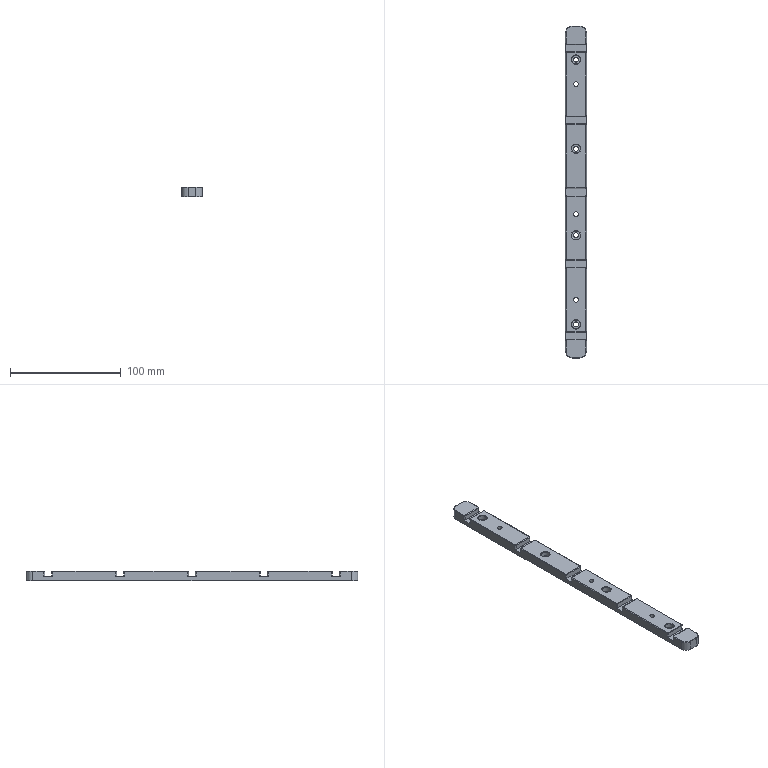CAM job | NX | 3-axis milling, drilling | part box 19 x 300 x 9 mm | stock box 20 x 305 x 12 mm
Tools:
number,name,description,diameter,corner_radius,flute_length,length,flutes
4,D4,平底铣刀-粗,4.0,0.0,25.0,75.0,2
6,D6,平底铣刀-粗,6.0,0.0,25.0,75.0,2
9,D10,平底铣刀-粗,10.0,0.0,35.0,75.0,2
7,D6-J,平底铣刀-精,6.0,0.0,25.0,75.0,2
17,D6R0.5,圆鼻刀-粗,6.0,0.5,50.0,75.0,2
1,D80R0.8飞刀,圆鼻刀-粗,80.0,0.8,50.0,75.0,2
1,D80R0.8飞刀-J,圆鼻刀-精,80.0,0.8,50.0,75.0,2
2,D6倒角刀,倒角刀,6.0,0.0,3.0,25.0,2
22,M5X0.8,丝锥,4.2,0.0,35.0,50.0,2
14,ZT4.2,钻头,4.2,0.0,35.0,50.0,2
11,ZT4.5,钻头,4.5,0.0,35.0,50.0,2
Operations:
program,operation,operation_type,tool,method,geometry_group,spindle_rpm,surface_speed,feed_per_tooth,feed_cut,feed_plunge,cut_length_mm,path_length_mm,cut_time_min,machine_time_min
B,底壁铣飞面一刀开粗_COPY,VolumeBased25DMillingOperation,D80R0.8飞刀,分层开粗-切深K-步距G,W-B,2800.0,703.696,0.5357,3000.0,100.0,2449.375,4573.571,0.8165,1.029
B,底壁铣飞面一刀精光_COPY,VolumeBased25DMillingOperation,D80R0.8飞刀-J,侧刃精光-切深K-步距G,W-B,4000.0,1005.28,0.125,1000.0,100.0,408.033,444.033,0.408,0.4116
B,钻倒角_1,Operation,D6倒角刀,METHOD,W-B,8000.0,150.796,0.0625,1000.0,0.0,17.1,275.296,0.0171,0.0429
B,钻倒角_2,Operation,D6倒角刀,METHOD,W-B,8000.0,150.796,0.0625,1000.0,0.0,22.2,332.769,0.0222,0.0533
B,C0.3封闭铣廓倒角6X45L_COPY,PlanarMilling,D6倒角刀,爬面_倒角-切深0-步距G,W-B,7000.0,131.0,0.1071,1500.0,100.0,645.331,681.331,0.4302,0.4338
A,顶面,FaceMilling,D80R0.8飞刀,侧刃精光-切深K-步距G,W-A,5000.0,1256.637,0.1,1000.0,100.0,394.0,430.0,0.394,0.3976
A,外形粗_2,VolumeBased25DMillingOperation,D10,METHOD,W-A,8000.0,251.327,0.3125,5000.0,80.0,9237.913,9285.713,1.848,1.852
A,底壁粗_1,VolumeBased25DMillingOperation,D6,METHOD,W-A,6000.0,113.0,0.2083,3500.0,100.0,2938.502,3787.114,0.8396,0.9244
A,打点-深0.8,Operation,D6倒角刀,NONE,W-A,8000.0,150.796,0.0312,500.0,90.0,12.6,310.497,0.0252,0.055
A,通孔-M5螺纹底孔,Operation,ZT4.2,NONE,W-A,3000.0,39.584,0.0583,350.0,90.0,51.785,340.582,0.148,0.1768
A,沉头孔-钻孔0段,Operation,ZT4.5,NONE,W-A,2800.0,39.584,0.0357,200.0,90.0,53.408,389.034,0.267,0.3006
A,铣孔开粗D4_1,CylinderMilling,D4,NONE,W-A,8000.0,100.531,0.075,1200.0,100.0,822.787,1316.587,0.6857,0.735
A,铣孔精光D4_1,CylinderMilling,D4,精光步距切深关,W-A,8000.0,100.531,0.0312,500.0,100.0,118.862,612.662,0.2377,0.2871
A,等高螺旋爬面_COPY,ZLevelMilling,D6R0.5,等高爬面-切深K-步距G,W-A,7000.0,131.947,0.3214,4500.0,100.0,14610.548,15355.567,3.247,3.321
A,铣倒角_1,PlanarMilling,D6倒角刀,METHOD,W-A,8000.0,150.796,0.0312,500.0,100.0,54.061,373.449,0.1081,0.1401
A,铣倒角_2,PlanarMilling,D6倒角刀,NONE,W-A,8000.0,150.796,0.0312,500.0,100.0,127.896,518.194,0.2558,0.2948
A,通孔-攻牙M5,Operation,M5X0.8,METHOD,W-A,500.0,6.597,0.0008,0.8,90.0,40.5,318.011,50.625,50.653
A,底侧精_3,VolumeBased25DMillingOperation,D6-J,METHOD,W-A,6000.0,113.0,0.2083,1200.0,100.0,393.08,1154.78,0.3276,0.4037
A,外形半精_2,VolumeBased25DMillingOperation,D6-J,METHOD,W-A,8000.0,251.327,0.0625,1000.0,100.0,651.54,709.14,0.6515,0.6573